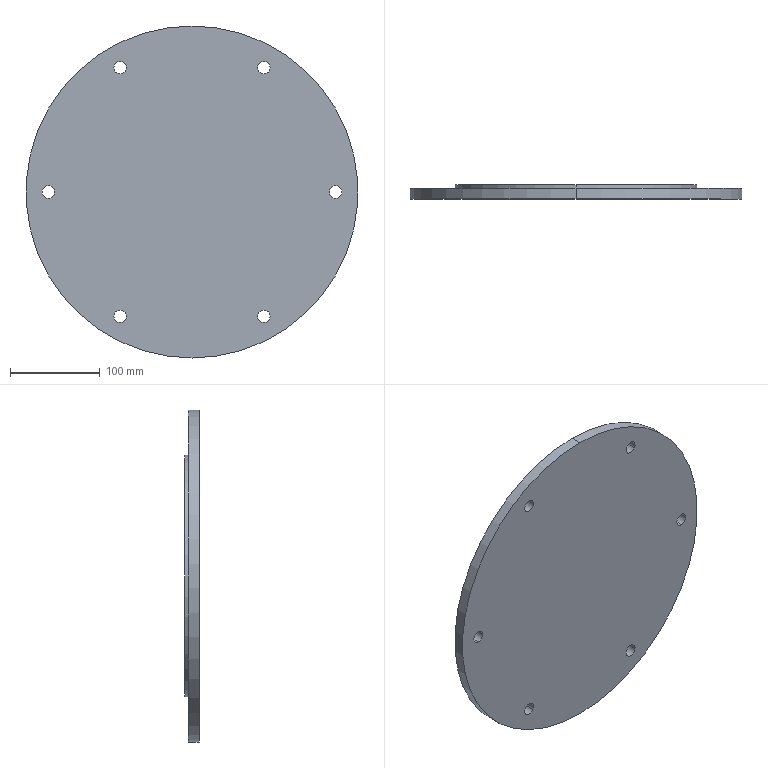Part | SolidWorks | features ICE 3, CirPattern 1, Extrusion 1 | 1 solid | 22 faces | box 370 x 16 x 370 mm | volume 1084232 mm3 | cylinder 18 | plane 4 | commonest cylinder face diameters 14 x12 259.5 x2 269.5 x2 370 x2
STEP:
#1=CARTESIAN_POINT('',(86.062,0.,135.064));
#2=VERTEX_POINT('',#1);
#3=CARTESIAN_POINT('',(73.938,0.,142.064));
#4=VERTEX_POINT('',#3);
#5=CARTESIAN_POINT('',(80.,0.,138.564));
#6=DIRECTION('',(0.,1.,0.));
#7=DIRECTION('',(-0.866,0.,0.5));
#8=AXIS2_PLACEMENT_3D('',#5,#6,#7);
#9=CIRCLE('',#8,7.);
#10=EDGE_CURVE('',#2,#4,#9,.T.);
#11=ORIENTED_EDGE('',*,*,#10,.F.);
#12=CARTESIAN_POINT('',(86.062,12.,135.064));
#13=VERTEX_POINT('',#12);
#14=CARTESIAN_POINT('',(86.062,0.,135.064));
#15=DIRECTION('',(0.,1.,0.));
#16=VECTOR('',#15,1000.);
#17=LINE('',#14,#16);
#18=EDGE_CURVE('',#2,#13,#17,.T.);
#19=ORIENTED_EDGE('',*,*,#18,.T.);
#20=CARTESIAN_POINT('',(73.938,12.,142.064));
#21=VERTEX_POINT('',#20);
#22=CARTESIAN_POINT('',(80.,12.,138.564));
#23=DIRECTION('',(0.,1.,0.));
#24=DIRECTION('',(-0.866,0.,0.5));
#25=AXIS2_PLACEMENT_3D('',#22,#23,#24);
#26=CIRCLE('',#25,7.);
#27=EDGE_CURVE('',#13,#21,#26,.T.);
#28=ORIENTED_EDGE('',*,*,#27,.T.);
#29=CARTESIAN_POINT('',(73.938,0.,142.064));
#30=DIRECTION('',(0.,1.,0.));
#31=VECTOR('',#30,1000.);
#32=LINE('',#29,#31);
#33=EDGE_CURVE('',#4,#21,#32,.T.);
#34=ORIENTED_EDGE('',*,*,#33,.F.);
#35=EDGE_LOOP('',(#11,#19,#28,#34));
#36=FACE_OUTER_BOUND('',#35,.T.);
#37=CARTESIAN_POINT('',(80.,0.,138.564));
#38=DIRECTION('',(0.,1.,0.));
#39=DIRECTION('',(-0.866,0.,0.5));
#40=AXIS2_PLACEMENT_3D('',#37,#38,#39);
#41=CYLINDRICAL_SURFACE('',#40,7.);
#42=ADVANCED_FACE('',(#36),#41,.F.);
#43=CARTESIAN_POINT('',(-73.938,0.,142.064));
#44=VERTEX_POINT('',#43);
#45=CARTESIAN_POINT('',(-86.062,0.,135.064));
#46=VERTEX_POINT('',#45);
#47=CARTESIAN_POINT('',(-80.,0.,138.564));
#48=DIRECTION('',(0.,1.,0.));
#49=DIRECTION('',(-0.866,0.,-0.5));
#50=AXIS2_PLACEMENT_3D('',#47,#48,#49);
#51=CIRCLE('',#50,7.);
#52=EDGE_CURVE('',#44,#46,#51,.T.);
#53=ORIENTED_EDGE('',*,*,#52,.F.);
#54=CARTESIAN_POINT('',(-73.938,12.,142.064));
#55=VERTEX_POINT('',#54);
#56=CARTESIAN_POINT('',(-73.938,0.,142.064));
#57=DIRECTION('',(0.,1.,0.));
#58=VECTOR('',#57,1000.);
#59=LINE('',#56,#58);
#60=EDGE_CURVE('',#44,#55,#59,.T.);
#61=ORIENTED_EDGE('',*,*,#60,.T.);
#62=CARTESIAN_POINT('',(-86.062,12.,135.064));
#63=VERTEX_POINT('',#62);
#64=CARTESIAN_POINT('',(-80.,12.,138.564));
#65=DIRECTION('',(0.,1.,0.));
#66=DIRECTION('',(-0.866,0.,-0.5));
#67=AXIS2_PLACEMENT_3D('',#64,#65,#66);
#68=CIRCLE('',#67,7.);
#69=EDGE_CURVE('',#55,#63,#68,.T.);
#70=ORIENTED_EDGE('',*,*,#69,.T.);
#71=CARTESIAN_POINT('',(-86.062,0.,135.064));
#72=DIRECTION('',(0.,1.,0.));
#73=VECTOR('',#72,1000.);
#74=LINE('',#71,#73);
#75=EDGE_CURVE('',#46,#63,#74,.T.);
#76=ORIENTED_EDGE('',*,*,#75,.F.);
#77=EDGE_LOOP('',(#53,#61,#70,#76));
#78=FACE_OUTER_BOUND('',#77,.T.);
#79=CARTESIAN_POINT('',(-80.,0.,138.564));
#80=DIRECTION('',(0.,1.,0.));
#81=DIRECTION('',(-0.866,0.,-0.5));
#82=AXIS2_PLACEMENT_3D('',#79,#80,#81);
#83=CYLINDRICAL_SURFACE('',#82,7.);
#84=ADVANCED_FACE('',(#78),#83,.F.);
#85=CARTESIAN_POINT('',(-160.,0.,7.));
#86=VERTEX_POINT('',#85);
#87=CARTESIAN_POINT('',(-160.,0.,-7.));
#88=VERTEX_POINT('',#87);
#89=CARTESIAN_POINT('',(-160.,0.,0.));
#90=DIRECTION('',(0.,1.,0.));
#91=DIRECTION('',(0.,0.,-1.));
#92=AXIS2_PLACEMENT_3D('',#89,#90,#91);
#93=CIRCLE('',#92,7.);
#94=EDGE_CURVE('',#86,#88,#93,.T.);
#95=ORIENTED_EDGE('',*,*,#94,.F.);
#96=CARTESIAN_POINT('',(-160.,12.,7.));
#97=VERTEX_POINT('',#96);
#98=CARTESIAN_POINT('',(-160.,0.,7.));
#99=DIRECTION('',(0.,1.,0.));
#100=VECTOR('',#99,1000.);
#101=LINE('',#98,#100);
#102=EDGE_CURVE('',#86,#97,#101,.T.);
#103=ORIENTED_EDGE('',*,*,#102,.T.);
#104=CARTESIAN_POINT('',(-160.,12.,-7.));
#105=VERTEX_POINT('',#104);
#106=CARTESIAN_POINT('',(-160.,12.,0.));
#107=DIRECTION('',(0.,1.,0.));
#108=DIRECTION('',(0.,0.,-1.));
#109=AXIS2_PLACEMENT_3D('',#106,#107,#108);
#110=CIRCLE('',#109,7.);
#111=EDGE_CURVE('',#97,#105,#110,.T.);
#112=ORIENTED_EDGE('',*,*,#111,.T.);
#113=CARTESIAN_POINT('',(-160.,0.,-7.));
#114=DIRECTION('',(0.,1.,0.));
#115=VECTOR('',#114,1000.);
#116=LINE('',#113,#115);
#117=EDGE_CURVE('',#88,#105,#116,.T.);
#118=ORIENTED_EDGE('',*,*,#117,.F.);
#119=EDGE_LOOP('',(#95,#103,#112,#118));
#120=FACE_OUTER_BOUND('',#119,.T.);
#121=CARTESIAN_POINT('',(-160.,0.,0.));
#122=DIRECTION('',(0.,1.,0.));
#123=DIRECTION('',(0.,0.,-1.));
#124=AXIS2_PLACEMENT_3D('',#121,#122,#123);
#125=CYLINDRICAL_SURFACE('',#124,7.);
#126=ADVANCED_FACE('',(#120),#125,.F.);
#127=CARTESIAN_POINT('',(-86.062,0.,-135.064));
#128=VERTEX_POINT('',#127);
#129=CARTESIAN_POINT('',(-73.938,0.,-142.064));
#130=VERTEX_POINT('',#129);
#131=CARTESIAN_POINT('',(-80.,0.,-138.564));
#132=DIRECTION('',(0.,1.,0.));
#133=DIRECTION('',(0.866,0.,-0.5));
#134=AXIS2_PLACEMENT_3D('',#131,#132,#133);
#135=CIRCLE('',#134,7.);
#136=EDGE_CURVE('',#128,#130,#135,.T.);
#137=ORIENTED_EDGE('',*,*,#136,.F.);
#138=CARTESIAN_POINT('',(-86.062,12.,-135.064));
#139=VERTEX_POINT('',#138);
#140=CARTESIAN_POINT('',(-86.062,0.,-135.064));
#141=DIRECTION('',(0.,1.,0.));
#142=VECTOR('',#141,1000.);
#143=LINE('',#140,#142);
#144=EDGE_CURVE('',#128,#139,#143,.T.);
#145=ORIENTED_EDGE('',*,*,#144,.T.);
#146=CARTESIAN_POINT('',(-73.938,12.,-142.064));
#147=VERTEX_POINT('',#146);
#148=CARTESIAN_POINT('',(-80.,12.,-138.564));
#149=DIRECTION('',(0.,1.,0.));
#150=DIRECTION('',(0.866,0.,-0.5));
#151=AXIS2_PLACEMENT_3D('',#148,#149,#150);
#152=CIRCLE('',#151,7.);
#153=EDGE_CURVE('',#139,#147,#152,.T.);
#154=ORIENTED_EDGE('',*,*,#153,.T.);
#155=CARTESIAN_POINT('',(-73.938,0.,-142.064));
#156=DIRECTION('',(0.,1.,0.));
#157=VECTOR('',#156,1000.);
#158=LINE('',#155,#157);
#159=EDGE_CURVE('',#130,#147,#158,.T.);
#160=ORIENTED_EDGE('',*,*,#159,.F.);
#161=EDGE_LOOP('',(#137,#145,#154,#160));
#162=FACE_OUTER_BOUND('',#161,.T.);
#163=CARTESIAN_POINT('',(-80.,0.,-138.564));
#164=DIRECTION('',(0.,1.,0.));
#165=DIRECTION('',(0.866,0.,-0.5));
#166=AXIS2_PLACEMENT_3D('',#163,#164,#165);
#167=CYLINDRICAL_SURFACE('',#166,7.);
#168=ADVANCED_FACE('',(#162),#167,.F.);
#169=CARTESIAN_POINT('',(73.938,0.,-142.064));
#170=VERTEX_POINT('',#169);
#171=CARTESIAN_POINT('',(86.062,0.,-135.064));
#172=VERTEX_POINT('',#171);
#173=CARTESIAN_POINT('',(80.,0.,-138.564));
#174=DIRECTION('',(0.,1.,0.));
#175=DIRECTION('',(0.866,0.,0.5));
#176=AXIS2_PLACEMENT_3D('',#173,#174,#175);
#177=CIRCLE('',#176,7.);
#178=EDGE_CURVE('',#170,#172,#177,.T.);
#179=ORIENTED_EDGE('',*,*,#178,.F.);
#180=CARTESIAN_POINT('',(73.938,12.,-142.064));
#181=VERTEX_POINT('',#180);
#182=CARTESIAN_POINT('',(73.938,0.,-142.064));
#183=DIRECTION('',(0.,1.,0.));
#184=VECTOR('',#183,1000.);
#185=LINE('',#182,#184);
#186=EDGE_CURVE('',#170,#181,#185,.T.);
#187=ORIENTED_EDGE('',*,*,#186,.T.);
#188=CARTESIAN_POINT('',(86.062,12.,-135.064));
#189=VERTEX_POINT('',#188);
#190=CARTESIAN_POINT('',(80.,12.,-138.564));
#191=DIRECTION('',(0.,1.,0.));
#192=DIRECTION('',(0.866,0.,0.5));
#193=AXIS2_PLACEMENT_3D('',#190,#191,#192);
#194=CIRCLE('',#193,7.);
#195=EDGE_CURVE('',#181,#189,#194,.T.);
#196=ORIENTED_EDGE('',*,*,#195,.T.);
#197=CARTESIAN_POINT('',(86.062,0.,-135.064));
#198=DIRECTION('',(0.,1.,0.));
#199=VECTOR('',#198,1000.);
#200=LINE('',#197,#199);
#201=EDGE_CURVE('',#172,#189,#200,.T.);
#202=ORIENTED_EDGE('',*,*,#201,.F.);
#203=EDGE_LOOP('',(#179,#187,#196,#202));
#204=FACE_OUTER_BOUND('',#203,.T.);
#205=CARTESIAN_POINT('',(80.,0.,-138.564));
#206=DIRECTION('',(0.,1.,0.));
#207=DIRECTION('',(0.866,0.,0.5));
#208=AXIS2_PLACEMENT_3D('',#205,#206,#207);
#209=CYLINDRICAL_SURFACE('',#208,7.);
#210=ADVANCED_FACE('',(#204),#209,.F.);
#211=CARTESIAN_POINT('',(160.,0.,-7.));
#212=VERTEX_POINT('',#211);
#213=CARTESIAN_POINT('',(160.,0.,7.));
#214=VERTEX_POINT('',#213);
#215=CARTESIAN_POINT('',(160.,0.,0.));
#216=DIRECTION('',(0.,1.,0.));
#217=DIRECTION('',(0.,0.,1.));
#218=AXIS2_PLACEMENT_3D('',#215,#216,#217);
#219=CIRCLE('',#218,7.);
#220=EDGE_CURVE('',#212,#214,#219,.T.);
#221=ORIENTED_EDGE('',*,*,#220,.F.);
#222=CARTESIAN_POINT('',(160.,12.,-7.));
#223=VERTEX_POINT('',#222);
#224=CARTESIAN_POINT('',(160.,0.,-7.));
#225=DIRECTION('',(0.,1.,0.));
#226=VECTOR('',#225,1000.);
#227=LINE('',#224,#226);
#228=EDGE_CURVE('',#212,#223,#227,.T.);
#229=ORIENTED_EDGE('',*,*,#228,.T.);
#230=CARTESIAN_POINT('',(160.,12.,7.));
#231=VERTEX_POINT('',#230);
#232=CARTESIAN_POINT('',(160.,12.,0.));
#233=DIRECTION('',(0.,1.,0.));
#234=DIRECTION('',(0.,0.,1.));
#235=AXIS2_PLACEMENT_3D('',#232,#233,#234);
#236=CIRCLE('',#235,7.);
#237=EDGE_CURVE('',#223,#231,#236,.T.);
#238=ORIENTED_EDGE('',*,*,#237,.T.);
#239=CARTESIAN_POINT('',(160.,0.,7.));
#240=DIRECTION('',(0.,1.,0.));
#241=VECTOR('',#240,1000.);
#242=LINE('',#239,#241);
#243=EDGE_CURVE('',#214,#231,#242,.T.);
#244=ORIENTED_EDGE('',*,*,#243,.F.);
#245=EDGE_LOOP('',(#221,#229,#238,#244));
#246=FACE_OUTER_BOUND('',#245,.T.);
#247=CARTESIAN_POINT('',(160.,0.,0.));
#248=DIRECTION('',(0.,1.,0.));
#249=DIRECTION('',(0.,0.,1.));
#250=AXIS2_PLACEMENT_3D('',#247,#248,#249);
#251=CYLINDRICAL_SURFACE('',#250,7.);
#252=ADVANCED_FACE('',(#246),#251,.F.);
#253=CARTESIAN_POINT('',(0.,8.,-129.75));
#254=VERTEX_POINT('',#253);
#255=CARTESIAN_POINT('',(0.,8.,129.75));
#256=VERTEX_POINT('',#255);
#257=CARTESIAN_POINT('',(0.,8.,0.));
#258=DIRECTION('',(0.,1.,0.));
#259=DIRECTION('',(0.,0.,1.));
#260=AXIS2_PLACEMENT_3D('',#257,#258,#259);
#261=CIRCLE('',#260,129.75);
#262=EDGE_CURVE('',#254,#256,#261,.T.);
#263=ORIENTED_EDGE('',*,*,#262,.F.);
#264=CARTESIAN_POINT('',(0.,16.,-129.75));
#265=VERTEX_POINT('',#264);
#266=CARTESIAN_POINT('',(0.,8.,-129.75));
#267=DIRECTION('',(0.,1.,0.));
#268=VECTOR('',#267,1000.);
#269=LINE('',#266,#268);
#270=EDGE_CURVE('',#254,#265,#269,.T.);
#271=ORIENTED_EDGE('',*,*,#270,.T.);
#272=CARTESIAN_POINT('',(0.,16.,129.75));
#273=VERTEX_POINT('',#272);
#274=CARTESIAN_POINT('',(0.,16.,0.));
#275=DIRECTION('',(0.,1.,0.));
#276=DIRECTION('',(0.,0.,1.));
#277=AXIS2_PLACEMENT_3D('',#274,#275,#276);
#278=CIRCLE('',#277,129.75);
#279=EDGE_CURVE('',#265,#273,#278,.T.);
#280=ORIENTED_EDGE('',*,*,#279,.T.);
#281=CARTESIAN_POINT('',(0.,8.,129.75));
#282=DIRECTION('',(0.,1.,0.));
#283=VECTOR('',#282,1000.);
#284=LINE('',#281,#283);
#285=EDGE_CURVE('',#256,#273,#284,.T.);
#286=ORIENTED_EDGE('',*,*,#285,.F.);
#287=EDGE_LOOP('',(#263,#271,#280,#286));
#288=FACE_OUTER_BOUND('',#287,.T.);
#289=CARTESIAN_POINT('',(0.,8.,0.));
#290=DIRECTION('',(0.,1.,0.));
#291=DIRECTION('',(0.,0.,1.));
#292=AXIS2_PLACEMENT_3D('',#289,#290,#291);
#293=CYLINDRICAL_SURFACE('',#292,129.75);
#294=ADVANCED_FACE('',(#288),#293,.F.);
#295=CARTESIAN_POINT('',(0.,16.,134.75));
#296=VERTEX_POINT('',#295);
#297=CARTESIAN_POINT('',(0.,16.,-134.75));
#298=VERTEX_POINT('',#297);
#299=CARTESIAN_POINT('',(0.,16.,0.));
#300=DIRECTION('',(0.,1.,0.));
#301=DIRECTION('',(0.,0.,1.));
#302=AXIS2_PLACEMENT_3D('',#299,#300,#301);
#303=CIRCLE('',#302,134.75);
#304=EDGE_CURVE('',#296,#298,#303,.T.);
#305=ORIENTED_EDGE('',*,*,#304,.F.);
#306=CARTESIAN_POINT('',(0.,12.,134.75));
#307=VERTEX_POINT('',#306);
#308=CARTESIAN_POINT('',(0.,16.,134.75));
#309=DIRECTION('',(0.,-1.,0.));
#310=VECTOR('',#309,1000.);
#311=LINE('',#308,#310);
#312=EDGE_CURVE('',#296,#307,#311,.T.);
#313=ORIENTED_EDGE('',*,*,#312,.T.);
#314=CARTESIAN_POINT('',(0.,12.,-134.75));
#315=VERTEX_POINT('',#314);
#316=CARTESIAN_POINT('',(0.,12.,0.));
#317=DIRECTION('',(0.,1.,0.));
#318=DIRECTION('',(0.,0.,1.));
#319=AXIS2_PLACEMENT_3D('',#316,#317,#318);
#320=CIRCLE('',#319,134.75);
#321=EDGE_CURVE('',#307,#315,#320,.T.);
#322=ORIENTED_EDGE('',*,*,#321,.T.);
#323=CARTESIAN_POINT('',(0.,16.,-134.75));
#324=DIRECTION('',(0.,-1.,0.));
#325=VECTOR('',#324,1000.);
#326=LINE('',#323,#325);
#327=EDGE_CURVE('',#298,#315,#326,.T.);
#328=ORIENTED_EDGE('',*,*,#327,.F.);
#329=EDGE_LOOP('',(#305,#313,#322,#328));
#330=FACE_OUTER_BOUND('',#329,.T.);
#331=CARTESIAN_POINT('',(0.,16.,0.));
#332=DIRECTION('',(0.,-1.,0.));
#333=DIRECTION('',(0.,0.,-1.));
#334=AXIS2_PLACEMENT_3D('',#331,#332,#333);
#335=CYLINDRICAL_SURFACE('',#334,134.75);
#336=ADVANCED_FACE('',(#330),#335,.T.);
#337=CARTESIAN_POINT('',(0.,12.,185.));
#338=VERTEX_POINT('',#337);
#339=CARTESIAN_POINT('',(0.,12.,-185.));
#340=VERTEX_POINT('',#339);
#341=CARTESIAN_POINT('',(0.,12.,0.));
#342=DIRECTION('',(0.,1.,0.));
#343=DIRECTION('',(0.,0.,1.));
#344=AXIS2_PLACEMENT_3D('',#341,#342,#343);
#345=CIRCLE('',#344,185.);
#346=EDGE_CURVE('',#338,#340,#345,.T.);
#347=ORIENTED_EDGE('',*,*,#346,.F.);
#348=CARTESIAN_POINT('',(0.,0.,185.));
#349=VERTEX_POINT('',#348);
#350=CARTESIAN_POINT('',(0.,12.,185.));
#351=DIRECTION('',(0.,-1.,0.));
#352=VECTOR('',#351,1000.);
#353=LINE('',#350,#352);
#354=EDGE_CURVE('',#338,#349,#353,.T.);
#355=ORIENTED_EDGE('',*,*,#354,.T.);
#356=CARTESIAN_POINT('',(0.,0.,-185.));
#357=VERTEX_POINT('',#356);
#358=CARTESIAN_POINT('',(0.,0.,0.));
#359=DIRECTION('',(0.,1.,0.));
#360=DIRECTION('',(0.,0.,1.));
#361=AXIS2_PLACEMENT_3D('',#358,#359,#360);
#362=CIRCLE('',#361,185.);
#363=EDGE_CURVE('',#349,#357,#362,.T.);
#364=ORIENTED_EDGE('',*,*,#363,.T.);
#365=CARTESIAN_POINT('',(0.,12.,-185.));
#366=DIRECTION('',(0.,-1.,0.));
#367=VECTOR('',#366,1000.);
#368=LINE('',#365,#367);
#369=EDGE_CURVE('',#340,#357,#368,.T.);
#370=ORIENTED_EDGE('',*,*,#369,.F.);
#371=EDGE_LOOP('',(#347,#355,#364,#370));
#372=FACE_OUTER_BOUND('',#371,.T.);
#373=CARTESIAN_POINT('',(0.,12.,0.));
#374=DIRECTION('',(0.,-1.,0.));
#375=DIRECTION('',(0.,0.,-1.));
#376=AXIS2_PLACEMENT_3D('',#373,#374,#375);
#377=CYLINDRICAL_SURFACE('',#376,185.);
#378=ADVANCED_FACE('',(#372),#377,.T.);
#379=CARTESIAN_POINT('',(80.,12.,138.564));
#380=DIRECTION('',(0.,1.,0.));
#381=DIRECTION('',(-0.866,0.,0.5));
#382=AXIS2_PLACEMENT_3D('',#379,#380,#381);
#383=CIRCLE('',#382,7.);
#384=EDGE_CURVE('',#21,#13,#383,.T.);
#385=ORIENTED_EDGE('',*,*,#384,.F.);
#386=ORIENTED_EDGE('',*,*,#27,.F.);
#387=EDGE_LOOP('',(#385,#386));
#388=FACE_BOUND('',#387,.T.);
#389=CARTESIAN_POINT('',(-80.,12.,138.564));
#390=DIRECTION('',(0.,1.,0.));
#391=DIRECTION('',(-0.866,0.,-0.5));
#392=AXIS2_PLACEMENT_3D('',#389,#390,#391);
#393=CIRCLE('',#392,7.);
#394=EDGE_CURVE('',#63,#55,#393,.T.);
#395=ORIENTED_EDGE('',*,*,#394,.F.);
#396=ORIENTED_EDGE('',*,*,#69,.F.);
#397=EDGE_LOOP('',(#395,#396));
#398=FACE_BOUND('',#397,.T.);
#399=CARTESIAN_POINT('',(-160.,12.,0.));
#400=DIRECTION('',(0.,1.,0.));
#401=DIRECTION('',(0.,0.,-1.));
#402=AXIS2_PLACEMENT_3D('',#399,#400,#401);
#403=CIRCLE('',#402,7.);
#404=EDGE_CURVE('',#105,#97,#403,.T.);
#405=ORIENTED_EDGE('',*,*,#404,.F.);
#406=ORIENTED_EDGE('',*,*,#111,.F.);
#407=EDGE_LOOP('',(#405,#406));
#408=FACE_BOUND('',#407,.T.);
#409=CARTESIAN_POINT('',(-80.,12.,-138.564));
#410=DIRECTION('',(0.,1.,0.));
#411=DIRECTION('',(0.866,0.,-0.5));
#412=AXIS2_PLACEMENT_3D('',#409,#410,#411);
#413=CIRCLE('',#412,7.);
#414=EDGE_CURVE('',#147,#139,#413,.T.);
#415=ORIENTED_EDGE('',*,*,#414,.F.);
#416=ORIENTED_EDGE('',*,*,#153,.F.);
#417=EDGE_LOOP('',(#415,#416));
#418=FACE_BOUND('',#417,.T.);
#419=CARTESIAN_POINT('',(80.,12.,-138.564));
#420=DIRECTION('',(0.,1.,0.));
#421=DIRECTION('',(0.866,0.,0.5));
#422=AXIS2_PLACEMENT_3D('',#419,#420,#421);
#423=CIRCLE('',#422,7.);
#424=EDGE_CURVE('',#189,#181,#423,.T.);
#425=ORIENTED_EDGE('',*,*,#424,.F.);
#426=ORIENTED_EDGE('',*,*,#195,.F.);
#427=EDGE_LOOP('',(#425,#426));
#428=FACE_BOUND('',#427,.T.);
#429=CARTESIAN_POINT('',(160.,12.,0.));
#430=DIRECTION('',(0.,1.,0.));
#431=DIRECTION('',(0.,0.,1.));
#432=AXIS2_PLACEMENT_3D('',#429,#430,#431);
#433=CIRCLE('',#432,7.);
#434=EDGE_CURVE('',#231,#223,#433,.T.);
#435=ORIENTED_EDGE('',*,*,#434,.F.);
#436=ORIENTED_EDGE('',*,*,#237,.F.);
#437=EDGE_LOOP('',(#435,#436));
#438=FACE_BOUND('',#437,.T.);
#439=CARTESIAN_POINT('',(0.,12.,0.));
#440=DIRECTION('',(0.,1.,0.));
#441=DIRECTION('',(0.,0.,1.));
#442=AXIS2_PLACEMENT_3D('',#439,#440,#441);
#443=CIRCLE('',#442,185.);
#444=EDGE_CURVE('',#340,#338,#443,.T.);
#445=ORIENTED_EDGE('',*,*,#444,.T.);
#446=ORIENTED_EDGE('',*,*,#346,.T.);
#447=EDGE_LOOP('',(#445,#446));
#448=FACE_OUTER_BOUND('',#447,.T.);
#449=CARTESIAN_POINT('',(0.,12.,0.));
#450=DIRECTION('',(0.,1.,0.));
#451=DIRECTION('',(0.,0.,1.));
#452=AXIS2_PLACEMENT_3D('',#449,#450,#451);
#453=CIRCLE('',#452,134.75);
#454=EDGE_CURVE('',#315,#307,#453,.T.);
#455=ORIENTED_EDGE('',*,*,#454,.F.);
#456=ORIENTED_EDGE('',*,*,#321,.F.);
#457=EDGE_LOOP('',(#455,#456));
#458=FACE_BOUND('',#457,.T.);
#459=CARTESIAN_POINT('',(0.,12.,0.));
#460=DIRECTION('',(0.,1.,0.));
#461=DIRECTION('',(0.,0.,1.));
#462=AXIS2_PLACEMENT_3D('',#459,#460,#461);
#463=PLANE('',#462);
#464=ADVANCED_FACE('',(#388,#398,#408,#418,#428,#438,#448,#458),#463,.T.);
#465=ORIENTED_EDGE('',*,*,#354,.F.);
#466=ORIENTED_EDGE('',*,*,#444,.F.);
#467=ORIENTED_EDGE('',*,*,#369,.T.);
#468=CARTESIAN_POINT('',(0.,0.,0.));
#469=DIRECTION('',(0.,1.,0.));
#470=DIRECTION('',(0.,0.,1.));
#471=AXIS2_PLACEMENT_3D('',#468,#469,#470);
#472=CIRCLE('',#471,185.);
#473=EDGE_CURVE('',#357,#349,#472,.T.);
#474=ORIENTED_EDGE('',*,*,#473,.T.);
#475=EDGE_LOOP('',(#465,#466,#467,#474));
#476=FACE_OUTER_BOUND('',#475,.T.);
#477=CARTESIAN_POINT('',(0.,12.,0.));
#478=DIRECTION('',(0.,-1.,0.));
#479=DIRECTION('',(0.,0.,-1.));
#480=AXIS2_PLACEMENT_3D('',#477,#478,#479);
#481=CYLINDRICAL_SURFACE('',#480,185.);
#482=ADVANCED_FACE('',(#476),#481,.T.);
#483=CARTESIAN_POINT('',(80.,0.,138.564));
#484=DIRECTION('',(0.,1.,0.));
#485=DIRECTION('',(-0.866,0.,0.5));
#486=AXIS2_PLACEMENT_3D('',#483,#484,#485);
#487=CIRCLE('',#486,7.);
#488=EDGE_CURVE('',#4,#2,#487,.T.);
#489=ORIENTED_EDGE('',*,*,#488,.T.);
#490=ORIENTED_EDGE('',*,*,#10,.T.);
#491=EDGE_LOOP('',(#489,#490));
#492=FACE_BOUND('',#491,.T.);
#493=CARTESIAN_POINT('',(-80.,0.,138.564));
#494=DIRECTION('',(0.,1.,0.));
#495=DIRECTION('',(-0.866,0.,-0.5));
#496=AXIS2_PLACEMENT_3D('',#493,#494,#495);
#497=CIRCLE('',#496,7.);
#498=EDGE_CURVE('',#46,#44,#497,.T.);
#499=ORIENTED_EDGE('',*,*,#498,.T.);
#500=ORIENTED_EDGE('',*,*,#52,.T.);
#501=EDGE_LOOP('',(#499,#500));
#502=FACE_BOUND('',#501,.T.);
#503=CARTESIAN_POINT('',(-160.,0.,0.));
#504=DIRECTION('',(0.,1.,0.));
#505=DIRECTION('',(0.,0.,-1.));
#506=AXIS2_PLACEMENT_3D('',#503,#504,#505);
#507=CIRCLE('',#506,7.);
#508=EDGE_CURVE('',#88,#86,#507,.T.);
#509=ORIENTED_EDGE('',*,*,#508,.T.);
#510=ORIENTED_EDGE('',*,*,#94,.T.);
#511=EDGE_LOOP('',(#509,#510));
#512=FACE_BOUND('',#511,.T.);
#513=CARTESIAN_POINT('',(-80.,0.,-138.564));
#514=DIRECTION('',(0.,1.,0.));
#515=DIRECTION('',(0.866,0.,-0.5));
#516=AXIS2_PLACEMENT_3D('',#513,#514,#515);
#517=CIRCLE('',#516,7.);
#518=EDGE_CURVE('',#130,#128,#517,.T.);
#519=ORIENTED_EDGE('',*,*,#518,.T.);
#520=ORIENTED_EDGE('',*,*,#136,.T.);
#521=EDGE_LOOP('',(#519,#520));
#522=FACE_BOUND('',#521,.T.);
#523=CARTESIAN_POINT('',(80.,0.,-138.564));
#524=DIRECTION('',(0.,1.,0.));
#525=DIRECTION('',(0.866,0.,0.5));
#526=AXIS2_PLACEMENT_3D('',#523,#524,#525);
#527=CIRCLE('',#526,7.);
#528=EDGE_CURVE('',#172,#170,#527,.T.);
#529=ORIENTED_EDGE('',*,*,#528,.T.);
#530=ORIENTED_EDGE('',*,*,#178,.T.);
#531=EDGE_LOOP('',(#529,#530));
#532=FACE_BOUND('',#531,.T.);
#533=CARTESIAN_POINT('',(160.,0.,0.));
#534=DIRECTION('',(0.,1.,0.));
#535=DIRECTION('',(0.,0.,1.));
#536=AXIS2_PLACEMENT_3D('',#533,#534,#535);
#537=CIRCLE('',#536,7.);
#538=EDGE_CURVE('',#214,#212,#537,.T.);
#539=ORIENTED_EDGE('',*,*,#538,.T.);
#540=ORIENTED_EDGE('',*,*,#220,.T.);
#541=EDGE_LOOP('',(#539,#540));
#542=FACE_BOUND('',#541,.T.);
#543=ORIENTED_EDGE('',*,*,#473,.F.);
#544=ORIENTED_EDGE('',*,*,#363,.F.);
#545=EDGE_LOOP('',(#543,#544));
#546=FACE_OUTER_BOUND('',#545,.T.);
#547=CARTESIAN_POINT('',(0.,0.,0.));
#548=DIRECTION('',(0.,1.,0.));
#549=DIRECTION('',(0.,0.,1.));
#550=AXIS2_PLACEMENT_3D('',#547,#548,#549);
#551=PLANE('',#550);
#552=ADVANCED_FACE('',(#492,#502,#512,#522,#532,#542,#546),#551,.F.);
#553=CARTESIAN_POINT('',(0.,16.,0.));
#554=DIRECTION('',(0.,1.,0.));
#555=DIRECTION('',(0.,0.,1.));
#556=AXIS2_PLACEMENT_3D('',#553,#554,#555);
#557=CIRCLE('',#556,134.75);
#558=EDGE_CURVE('',#298,#296,#557,.T.);
#559=ORIENTED_EDGE('',*,*,#558,.T.);
#560=ORIENTED_EDGE('',*,*,#304,.T.);
#561=EDGE_LOOP('',(#559,#560));
#562=FACE_OUTER_BOUND('',#561,.T.);
#563=CARTESIAN_POINT('',(0.,16.,0.));
#564=DIRECTION('',(0.,1.,0.));
#565=DIRECTION('',(0.,0.,1.));
#566=AXIS2_PLACEMENT_3D('',#563,#564,#565);
#567=CIRCLE('',#566,129.75);
#568=EDGE_CURVE('',#273,#265,#567,.T.);
#569=ORIENTED_EDGE('',*,*,#568,.F.);
#570=ORIENTED_EDGE('',*,*,#279,.F.);
#571=EDGE_LOOP('',(#569,#570));
#572=FACE_BOUND('',#571,.T.);
#573=CARTESIAN_POINT('',(0.,16.,0.));
#574=DIRECTION('',(0.,1.,0.));
#575=DIRECTION('',(0.,0.,1.));
#576=AXIS2_PLACEMENT_3D('',#573,#574,#575);
#577=PLANE('',#576);
#578=ADVANCED_FACE('',(#562,#572),#577,.T.);
#579=ORIENTED_EDGE('',*,*,#312,.F.);
#580=ORIENTED_EDGE('',*,*,#558,.F.);
#581=ORIENTED_EDGE('',*,*,#327,.T.);
#582=ORIENTED_EDGE('',*,*,#454,.T.);
#583=EDGE_LOOP('',(#579,#580,#581,#582));
#584=FACE_OUTER_BOUND('',#583,.T.);
#585=CARTESIAN_POINT('',(0.,16.,0.));
#586=DIRECTION('',(0.,-1.,0.));
#587=DIRECTION('',(0.,0.,-1.));
#588=AXIS2_PLACEMENT_3D('',#585,#586,#587);
#589=CYLINDRICAL_SURFACE('',#588,134.75);
#590=ADVANCED_FACE('',(#584),#589,.T.);
#591=CARTESIAN_POINT('',(0.,8.,0.));
#592=DIRECTION('',(0.,1.,0.));
#593=DIRECTION('',(0.,0.,1.));
#594=AXIS2_PLACEMENT_3D('',#591,#592,#593);
#595=CIRCLE('',#594,129.75);
#596=EDGE_CURVE('',#256,#254,#595,.T.);
#597=ORIENTED_EDGE('',*,*,#596,.T.);
#598=ORIENTED_EDGE('',*,*,#262,.T.);
#599=EDGE_LOOP('',(#597,#598));
#600=FACE_OUTER_BOUND('',#599,.T.);
#601=CARTESIAN_POINT('',(0.,8.,0.));
#602=DIRECTION('',(0.,1.,0.));
#603=DIRECTION('',(0.,0.,1.));
#604=AXIS2_PLACEMENT_3D('',#601,#602,#603);
#605=PLANE('',#604);
#606=ADVANCED_FACE('',(#600),#605,.T.);
#607=ORIENTED_EDGE('',*,*,#270,.F.);
#608=ORIENTED_EDGE('',*,*,#596,.F.);
#609=ORIENTED_EDGE('',*,*,#285,.T.);
#610=ORIENTED_EDGE('',*,*,#568,.T.);
#611=EDGE_LOOP('',(#607,#608,#609,#610));
#612=FACE_OUTER_BOUND('',#611,.T.);
#613=CARTESIAN_POINT('',(0.,8.,0.));
#614=DIRECTION('',(0.,1.,0.));
#615=DIRECTION('',(0.,0.,1.));
#616=AXIS2_PLACEMENT_3D('',#613,#614,#615);
#617=CYLINDRICAL_SURFACE('',#616,129.75);
#618=ADVANCED_FACE('',(#612),#617,.F.);
#619=ORIENTED_EDGE('',*,*,#228,.F.);
#620=ORIENTED_EDGE('',*,*,#538,.F.);
#621=ORIENTED_EDGE('',*,*,#243,.T.);
#622=ORIENTED_EDGE('',*,*,#434,.T.);
#623=EDGE_LOOP('',(#619,#620,#621,#622));
#624=FACE_OUTER_BOUND('',#623,.T.);
#625=CARTESIAN_POINT('',(160.,0.,0.));
#626=DIRECTION('',(0.,1.,0.));
#627=DIRECTION('',(0.,0.,1.));
#628=AXIS2_PLACEMENT_3D('',#625,#626,#627);
#629=CYLINDRICAL_SURFACE('',#628,7.);
#630=ADVANCED_FACE('',(#624),#629,.F.);
#631=ORIENTED_EDGE('',*,*,#186,.F.);
#632=ORIENTED_EDGE('',*,*,#528,.F.);
#633=ORIENTED_EDGE('',*,*,#201,.T.);
#634=ORIENTED_EDGE('',*,*,#424,.T.);
#635=EDGE_LOOP('',(#631,#632,#633,#634));
#636=FACE_OUTER_BOUND('',#635,.T.);
#637=CARTESIAN_POINT('',(80.,0.,-138.564));
#638=DIRECTION('',(0.,1.,0.));
#639=DIRECTION('',(0.866,0.,0.5));
#640=AXIS2_PLACEMENT_3D('',#637,#638,#639);
#641=CYLINDRICAL_SURFACE('',#640,7.);
#642=ADVANCED_FACE('',(#636),#641,.F.);
#643=ORIENTED_EDGE('',*,*,#144,.F.);
#644=ORIENTED_EDGE('',*,*,#518,.F.);
#645=ORIENTED_EDGE('',*,*,#159,.T.);
#646=ORIENTED_EDGE('',*,*,#414,.T.);
#647=EDGE_LOOP('',(#643,#644,#645,#646));
#648=FACE_OUTER_BOUND('',#647,.T.);
#649=CARTESIAN_POINT('',(-80.,0.,-138.564));
#650=DIRECTION('',(0.,1.,0.));
#651=DIRECTION('',(0.866,0.,-0.5));
#652=AXIS2_PLACEMENT_3D('',#649,#650,#651);
#653=CYLINDRICAL_SURFACE('',#652,7.);
#654=ADVANCED_FACE('',(#648),#653,.F.);
#655=ORIENTED_EDGE('',*,*,#102,.F.);
#656=ORIENTED_EDGE('',*,*,#508,.F.);
#657=ORIENTED_EDGE('',*,*,#117,.T.);
#658=ORIENTED_EDGE('',*,*,#404,.T.);
#659=EDGE_LOOP('',(#655,#656,#657,#658));
#660=FACE_OUTER_BOUND('',#659,.T.);
#661=CARTESIAN_POINT('',(-160.,0.,0.));
#662=DIRECTION('',(0.,1.,0.));
#663=DIRECTION('',(0.,0.,-1.));
#664=AXIS2_PLACEMENT_3D('',#661,#662,#663);
#665=CYLINDRICAL_SURFACE('',#664,7.);
#666=ADVANCED_FACE('',(#660),#665,.F.);
#667=ORIENTED_EDGE('',*,*,#60,.F.);
#668=ORIENTED_EDGE('',*,*,#498,.F.);
#669=ORIENTED_EDGE('',*,*,#75,.T.);
#670=ORIENTED_EDGE('',*,*,#394,.T.);
#671=EDGE_LOOP('',(#667,#668,#669,#670));
#672=FACE_OUTER_BOUND('',#671,.T.);
#673=CARTESIAN_POINT('',(-80.,0.,138.564));
#674=DIRECTION('',(0.,1.,0.));
#675=DIRECTION('',(-0.866,0.,-0.5));
#676=AXIS2_PLACEMENT_3D('',#673,#674,#675);
#677=CYLINDRICAL_SURFACE('',#676,7.);
#678=ADVANCED_FACE('',(#672),#677,.F.);
#679=ORIENTED_EDGE('',*,*,#18,.F.);
#680=ORIENTED_EDGE('',*,*,#488,.F.);
#681=ORIENTED_EDGE('',*,*,#33,.T.);
#682=ORIENTED_EDGE('',*,*,#384,.T.);
#683=EDGE_LOOP('',(#679,#680,#681,#682));
#684=FACE_OUTER_BOUND('',#683,.T.);
#685=CARTESIAN_POINT('',(80.,0.,138.564));
#686=DIRECTION('',(0.,1.,0.));
#687=DIRECTION('',(-0.866,0.,0.5));
#688=AXIS2_PLACEMENT_3D('',#685,#686,#687);
#689=CYLINDRICAL_SURFACE('',#688,7.);
#690=ADVANCED_FACE('',(#684),#689,.F.);
#691=CLOSED_SHELL('',(#42,#84,#126,#168,#210,#252,#294,#336,#378,#464,#482,#552,#578,#590,#606,#618,#630,#642,#654,#666,#678,#690));
#692=MANIFOLD_SOLID_BREP('',#691);
#693=CARTESIAN_POINT('',(0.,0.,0.));
#694=DIRECTION('',(0.,0.,1.));
#695=DIRECTION('',(1.,0.,0.));
#696=AXIS2_PLACEMENT_3D('',#693,#694,#695);
#697=(LENGTH_UNIT()NAMED_UNIT(*)SI_UNIT(.MILLI.,.METRE.));
#698=UNCERTAINTY_MEASURE_WITH_UNIT(LENGTH_MEASURE(0.00001),#697,'','');
#699=(NAMED_UNIT(*)PLANE_ANGLE_UNIT()SI_UNIT($,.RADIAN.));
#700=(NAMED_UNIT(*)SI_UNIT($,.STERADIAN.)SOLID_ANGLE_UNIT());
#701=(GEOMETRIC_REPRESENTATION_CONTEXT(3)GLOBAL_UNCERTAINTY_ASSIGNED_CONTEXT((#698))GLOBAL_UNIT_ASSIGNED_CONTEXT((#697,#699,#700))REPRESENTATION_CONTEXT('',''));
#702=ADVANCED_BREP_SHAPE_REPRESENTATION('',(#692,#696),#701);